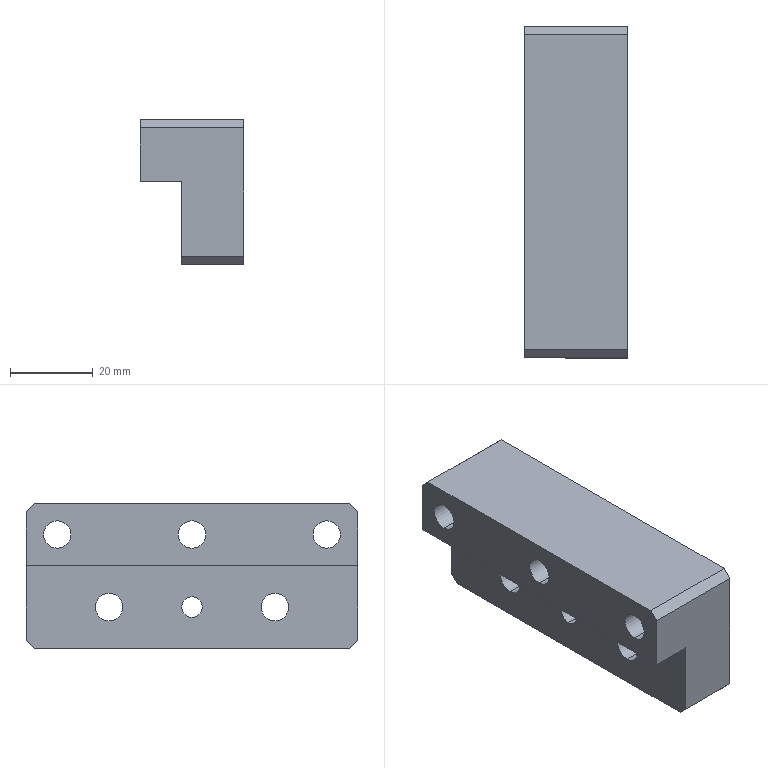Part | SolidWorks | features HoleWzd 3, Chamfer 1, Extrusion 1 | 1 solid | 39 faces | box 25 x 80 x 35 mm | volume 46243 mm3 | cylinder 22 | plane 17 | commonest cylinder face diameters 6.6 x10 11 x10 5 x2
STEP:
#1=CARTESIAN_POINT('',(17.,20.,-19.5));
#2=VERTEX_POINT('',#1);
#3=CARTESIAN_POINT('',(17.,20.,-30.5));
#4=VERTEX_POINT('',#3);
#5=CARTESIAN_POINT('',(17.,20.,-25.));
#6=DIRECTION('',(1.,0.,0.));
#7=DIRECTION('',(0.,0.,-1.));
#8=AXIS2_PLACEMENT_3D('',#5,#6,#7);
#9=CIRCLE('',#8,5.5);
#10=EDGE_CURVE('',#2,#4,#9,.T.);
#11=ORIENTED_EDGE('',*,*,#10,.F.);
#12=CARTESIAN_POINT('',(25.,20.,-19.5));
#13=VERTEX_POINT('',#12);
#14=CARTESIAN_POINT('',(25.,20.,-19.5));
#15=DIRECTION('',(1.,0.,0.));
#16=VECTOR('',#15,1000.);
#17=LINE('',#14,#16);
#18=EDGE_CURVE('',#2,#13,#17,.T.);
#19=ORIENTED_EDGE('',*,*,#18,.T.);
#20=CARTESIAN_POINT('',(25.,20.,-30.5));
#21=VERTEX_POINT('',#20);
#22=CARTESIAN_POINT('',(25.,20.,-25.));
#23=DIRECTION('',(1.,0.,0.));
#24=DIRECTION('',(0.,0.,-1.));
#25=AXIS2_PLACEMENT_3D('',#22,#23,#24);
#26=CIRCLE('',#25,5.5);
#27=EDGE_CURVE('',#13,#21,#26,.T.);
#28=ORIENTED_EDGE('',*,*,#27,.T.);
#29=CARTESIAN_POINT('',(25.,20.,-30.5));
#30=DIRECTION('',(1.,0.,0.));
#31=VECTOR('',#30,1000.);
#32=LINE('',#29,#31);
#33=EDGE_CURVE('',#4,#21,#32,.T.);
#34=ORIENTED_EDGE('',*,*,#33,.F.);
#35=EDGE_LOOP('',(#11,#19,#28,#34));
#36=FACE_OUTER_BOUND('',#35,.T.);
#37=CARTESIAN_POINT('',(25.,20.,-25.));
#38=DIRECTION('',(1.,0.,0.));
#39=DIRECTION('',(0.,0.,-1.));
#40=AXIS2_PLACEMENT_3D('',#37,#38,#39);
#41=CYLINDRICAL_SURFACE('',#40,5.5);
#42=ADVANCED_FACE('',(#36),#41,.F.);
#43=CARTESIAN_POINT('',(10.,20.,-21.7));
#44=VERTEX_POINT('',#43);
#45=CARTESIAN_POINT('',(10.,20.,-28.3));
#46=VERTEX_POINT('',#45);
#47=CARTESIAN_POINT('',(10.,20.,-25.));
#48=DIRECTION('',(1.,0.,0.));
#49=DIRECTION('',(0.,0.,-1.));
#50=AXIS2_PLACEMENT_3D('',#47,#48,#49);
#51=CIRCLE('',#50,3.3);
#52=EDGE_CURVE('',#44,#46,#51,.T.);
#53=ORIENTED_EDGE('',*,*,#52,.F.);
#54=CARTESIAN_POINT('',(17.,20.,-21.7));
#55=VERTEX_POINT('',#54);
#56=CARTESIAN_POINT('',(25.,20.,-21.7));
#57=DIRECTION('',(1.,0.,0.));
#58=VECTOR('',#57,1000.);
#59=LINE('',#56,#58);
#60=EDGE_CURVE('',#44,#55,#59,.T.);
#61=ORIENTED_EDGE('',*,*,#60,.T.);
#62=CARTESIAN_POINT('',(17.,20.,-28.3));
#63=VERTEX_POINT('',#62);
#64=CARTESIAN_POINT('',(17.,20.,-25.));
#65=DIRECTION('',(1.,0.,0.));
#66=DIRECTION('',(0.,0.,-1.));
#67=AXIS2_PLACEMENT_3D('',#64,#65,#66);
#68=CIRCLE('',#67,3.3);
#69=EDGE_CURVE('',#55,#63,#68,.T.);
#70=ORIENTED_EDGE('',*,*,#69,.T.);
#71=CARTESIAN_POINT('',(25.,20.,-28.3));
#72=DIRECTION('',(1.,0.,0.));
#73=VECTOR('',#72,1000.);
#74=LINE('',#71,#73);
#75=EDGE_CURVE('',#46,#63,#74,.T.);
#76=ORIENTED_EDGE('',*,*,#75,.F.);
#77=EDGE_LOOP('',(#53,#61,#70,#76));
#78=FACE_OUTER_BOUND('',#77,.T.);
#79=CARTESIAN_POINT('',(25.,20.,-25.));
#80=DIRECTION('',(1.,0.,0.));
#81=DIRECTION('',(0.,0.,-1.));
#82=AXIS2_PLACEMENT_3D('',#79,#80,#81);
#83=CYLINDRICAL_SURFACE('',#82,3.3);
#84=ADVANCED_FACE('',(#78),#83,.F.);
#85=CARTESIAN_POINT('',(17.,-20.,-19.5));
#86=VERTEX_POINT('',#85);
#87=CARTESIAN_POINT('',(17.,-20.,-30.5));
#88=VERTEX_POINT('',#87);
#89=CARTESIAN_POINT('',(17.,-20.,-25.));
#90=DIRECTION('',(1.,0.,0.));
#91=DIRECTION('',(0.,0.,-1.));
#92=AXIS2_PLACEMENT_3D('',#89,#90,#91);
#93=CIRCLE('',#92,5.5);
#94=EDGE_CURVE('',#86,#88,#93,.T.);
#95=ORIENTED_EDGE('',*,*,#94,.F.);
#96=CARTESIAN_POINT('',(25.,-20.,-19.5));
#97=VERTEX_POINT('',#96);
#98=CARTESIAN_POINT('',(25.,-20.,-19.5));
#99=DIRECTION('',(1.,0.,0.));
#100=VECTOR('',#99,1000.);
#101=LINE('',#98,#100);
#102=EDGE_CURVE('',#86,#97,#101,.T.);
#103=ORIENTED_EDGE('',*,*,#102,.T.);
#104=CARTESIAN_POINT('',(25.,-20.,-30.5));
#105=VERTEX_POINT('',#104);
#106=CARTESIAN_POINT('',(25.,-20.,-25.));
#107=DIRECTION('',(1.,0.,0.));
#108=DIRECTION('',(0.,0.,-1.));
#109=AXIS2_PLACEMENT_3D('',#106,#107,#108);
#110=CIRCLE('',#109,5.5);
#111=EDGE_CURVE('',#97,#105,#110,.T.);
#112=ORIENTED_EDGE('',*,*,#111,.T.);
#113=CARTESIAN_POINT('',(25.,-20.,-30.5));
#114=DIRECTION('',(1.,0.,0.));
#115=VECTOR('',#114,1000.);
#116=LINE('',#113,#115);
#117=EDGE_CURVE('',#88,#105,#116,.T.);
#118=ORIENTED_EDGE('',*,*,#117,.F.);
#119=EDGE_LOOP('',(#95,#103,#112,#118));
#120=FACE_OUTER_BOUND('',#119,.T.);
#121=CARTESIAN_POINT('',(25.,-20.,-25.));
#122=DIRECTION('',(1.,0.,0.));
#123=DIRECTION('',(0.,0.,-1.));
#124=AXIS2_PLACEMENT_3D('',#121,#122,#123);
#125=CYLINDRICAL_SURFACE('',#124,5.5);
#126=ADVANCED_FACE('',(#120),#125,.F.);
#127=CARTESIAN_POINT('',(10.,-20.,-21.7));
#128=VERTEX_POINT('',#127);
#129=CARTESIAN_POINT('',(10.,-20.,-28.3));
#130=VERTEX_POINT('',#129);
#131=CARTESIAN_POINT('',(10.,-20.,-25.));
#132=DIRECTION('',(1.,0.,0.));
#133=DIRECTION('',(0.,0.,-1.));
#134=AXIS2_PLACEMENT_3D('',#131,#132,#133);
#135=CIRCLE('',#134,3.3);
#136=EDGE_CURVE('',#128,#130,#135,.T.);
#137=ORIENTED_EDGE('',*,*,#136,.F.);
#138=CARTESIAN_POINT('',(17.,-20.,-21.7));
#139=VERTEX_POINT('',#138);
#140=CARTESIAN_POINT('',(25.,-20.,-21.7));
#141=DIRECTION('',(1.,0.,0.));
#142=VECTOR('',#141,1000.);
#143=LINE('',#140,#142);
#144=EDGE_CURVE('',#128,#139,#143,.T.);
#145=ORIENTED_EDGE('',*,*,#144,.T.);
#146=CARTESIAN_POINT('',(17.,-20.,-28.3));
#147=VERTEX_POINT('',#146);
#148=CARTESIAN_POINT('',(17.,-20.,-25.));
#149=DIRECTION('',(1.,0.,0.));
#150=DIRECTION('',(0.,0.,-1.));
#151=AXIS2_PLACEMENT_3D('',#148,#149,#150);
#152=CIRCLE('',#151,3.3);
#153=EDGE_CURVE('',#139,#147,#152,.T.);
#154=ORIENTED_EDGE('',*,*,#153,.T.);
#155=CARTESIAN_POINT('',(25.,-20.,-28.3));
#156=DIRECTION('',(1.,0.,0.));
#157=VECTOR('',#156,1000.);
#158=LINE('',#155,#157);
#159=EDGE_CURVE('',#130,#147,#158,.T.);
#160=ORIENTED_EDGE('',*,*,#159,.F.);
#161=EDGE_LOOP('',(#137,#145,#154,#160));
#162=FACE_OUTER_BOUND('',#161,.T.);
#163=CARTESIAN_POINT('',(25.,-20.,-25.));
#164=DIRECTION('',(1.,0.,0.));
#165=DIRECTION('',(0.,0.,-1.));
#166=AXIS2_PLACEMENT_3D('',#163,#164,#165);
#167=CYLINDRICAL_SURFACE('',#166,3.3);
#168=ADVANCED_FACE('',(#162),#167,.F.);
#169=CARTESIAN_POINT('',(10.,0.,-22.5));
#170=VERTEX_POINT('',#169);
#171=CARTESIAN_POINT('',(10.,0.,-27.5));
#172=VERTEX_POINT('',#171);
#173=CARTESIAN_POINT('',(10.,0.,-25.));
#174=DIRECTION('',(1.,0.,0.));
#175=DIRECTION('',(0.,0.,-1.));
#176=AXIS2_PLACEMENT_3D('',#173,#174,#175);
#177=CIRCLE('',#176,2.5);
#178=EDGE_CURVE('',#170,#172,#177,.T.);
#179=ORIENTED_EDGE('',*,*,#178,.F.);
#180=CARTESIAN_POINT('',(25.,0.,-22.5));
#181=VERTEX_POINT('',#180);
#182=CARTESIAN_POINT('',(25.,0.,-22.5));
#183=DIRECTION('',(1.,0.,0.));
#184=VECTOR('',#183,1000.);
#185=LINE('',#182,#184);
#186=EDGE_CURVE('',#170,#181,#185,.T.);
#187=ORIENTED_EDGE('',*,*,#186,.T.);
#188=CARTESIAN_POINT('',(25.,0.,-27.5));
#189=VERTEX_POINT('',#188);
#190=CARTESIAN_POINT('',(25.,0.,-25.));
#191=DIRECTION('',(1.,0.,0.));
#192=DIRECTION('',(0.,0.,-1.));
#193=AXIS2_PLACEMENT_3D('',#190,#191,#192);
#194=CIRCLE('',#193,2.5);
#195=EDGE_CURVE('',#181,#189,#194,.T.);
#196=ORIENTED_EDGE('',*,*,#195,.T.);
#197=CARTESIAN_POINT('',(25.,0.,-27.5));
#198=DIRECTION('',(1.,0.,0.));
#199=VECTOR('',#198,1000.);
#200=LINE('',#197,#199);
#201=EDGE_CURVE('',#172,#189,#200,.T.);
#202=ORIENTED_EDGE('',*,*,#201,.F.);
#203=EDGE_LOOP('',(#179,#187,#196,#202));
#204=FACE_OUTER_BOUND('',#203,.T.);
#205=CARTESIAN_POINT('',(25.,0.,-25.));
#206=DIRECTION('',(1.,0.,0.));
#207=DIRECTION('',(0.,0.,-1.));
#208=AXIS2_PLACEMENT_3D('',#205,#206,#207);
#209=CYLINDRICAL_SURFACE('',#208,2.5);
#210=ADVANCED_FACE('',(#204),#209,.F.);
#211=CARTESIAN_POINT('',(10.,32.5,-2.));
#212=VERTEX_POINT('',#211);
#213=CARTESIAN_POINT('',(10.,32.5,-13.));
#214=VERTEX_POINT('',#213);
#215=CARTESIAN_POINT('',(10.,32.5,-7.5));
#216=DIRECTION('',(1.,0.,0.));
#217=DIRECTION('',(0.,0.,-1.));
#218=AXIS2_PLACEMENT_3D('',#215,#216,#217);
#219=CIRCLE('',#218,5.5);
#220=EDGE_CURVE('',#212,#214,#219,.T.);
#221=ORIENTED_EDGE('',*,*,#220,.F.);
#222=CARTESIAN_POINT('',(25.,32.5,-2.));
#223=VERTEX_POINT('',#222);
#224=CARTESIAN_POINT('',(25.,32.5,-2.));
#225=DIRECTION('',(1.,0.,0.));
#226=VECTOR('',#225,1000.);
#227=LINE('',#224,#226);
#228=EDGE_CURVE('',#212,#223,#227,.T.);
#229=ORIENTED_EDGE('',*,*,#228,.T.);
#230=CARTESIAN_POINT('',(25.,32.5,-13.));
#231=VERTEX_POINT('',#230);
#232=CARTESIAN_POINT('',(25.,32.5,-7.5));
#233=DIRECTION('',(1.,0.,0.));
#234=DIRECTION('',(0.,0.,-1.));
#235=AXIS2_PLACEMENT_3D('',#232,#233,#234);
#236=CIRCLE('',#235,5.5);
#237=EDGE_CURVE('',#223,#231,#236,.T.);
#238=ORIENTED_EDGE('',*,*,#237,.T.);
#239=CARTESIAN_POINT('',(25.,32.5,-13.));
#240=DIRECTION('',(1.,0.,0.));
#241=VECTOR('',#240,1000.);
#242=LINE('',#239,#241);
#243=EDGE_CURVE('',#214,#231,#242,.T.);
#244=ORIENTED_EDGE('',*,*,#243,.F.);
#245=EDGE_LOOP('',(#221,#229,#238,#244));
#246=FACE_OUTER_BOUND('',#245,.T.);
#247=CARTESIAN_POINT('',(25.,32.5,-7.5));
#248=DIRECTION('',(1.,0.,0.));
#249=DIRECTION('',(0.,0.,-1.));
#250=AXIS2_PLACEMENT_3D('',#247,#248,#249);
#251=CYLINDRICAL_SURFACE('',#250,5.5);
#252=ADVANCED_FACE('',(#246),#251,.F.);
#253=CARTESIAN_POINT('',(0.,32.5,-4.2));
#254=VERTEX_POINT('',#253);
#255=CARTESIAN_POINT('',(0.,32.5,-10.8));
#256=VERTEX_POINT('',#255);
#257=CARTESIAN_POINT('',(0.,32.5,-7.5));
#258=DIRECTION('',(1.,0.,0.));
#259=DIRECTION('',(0.,0.,-1.));
#260=AXIS2_PLACEMENT_3D('',#257,#258,#259);
#261=CIRCLE('',#260,3.3);
#262=EDGE_CURVE('',#254,#256,#261,.T.);
#263=ORIENTED_EDGE('',*,*,#262,.F.);
#264=CARTESIAN_POINT('',(10.,32.5,-4.2));
#265=VERTEX_POINT('',#264);
#266=CARTESIAN_POINT('',(25.,32.5,-4.2));
#267=DIRECTION('',(1.,0.,0.));
#268=VECTOR('',#267,1000.);
#269=LINE('',#266,#268);
#270=EDGE_CURVE('',#254,#265,#269,.T.);
#271=ORIENTED_EDGE('',*,*,#270,.T.);
#272=CARTESIAN_POINT('',(10.,32.5,-10.8));
#273=VERTEX_POINT('',#272);
#274=CARTESIAN_POINT('',(10.,32.5,-7.5));
#275=DIRECTION('',(1.,0.,0.));
#276=DIRECTION('',(0.,0.,-1.));
#277=AXIS2_PLACEMENT_3D('',#274,#275,#276);
#278=CIRCLE('',#277,3.3);
#279=EDGE_CURVE('',#265,#273,#278,.T.);
#280=ORIENTED_EDGE('',*,*,#279,.T.);
#281=CARTESIAN_POINT('',(25.,32.5,-10.8));
#282=DIRECTION('',(1.,0.,0.));
#283=VECTOR('',#282,1000.);
#284=LINE('',#281,#283);
#285=EDGE_CURVE('',#256,#273,#284,.T.);
#286=ORIENTED_EDGE('',*,*,#285,.F.);
#287=EDGE_LOOP('',(#263,#271,#280,#286));
#288=FACE_OUTER_BOUND('',#287,.T.);
#289=CARTESIAN_POINT('',(25.,32.5,-7.5));
#290=DIRECTION('',(1.,0.,0.));
#291=DIRECTION('',(0.,0.,-1.));
#292=AXIS2_PLACEMENT_3D('',#289,#290,#291);
#293=CYLINDRICAL_SURFACE('',#292,3.3);
#294=ADVANCED_FACE('',(#288),#293,.F.);
#295=CARTESIAN_POINT('',(10.,0.,-2.));
#296=VERTEX_POINT('',#295);
#297=CARTESIAN_POINT('',(10.,0.,-13.));
#298=VERTEX_POINT('',#297);
#299=CARTESIAN_POINT('',(10.,0.,-7.5));
#300=DIRECTION('',(1.,0.,0.));
#301=DIRECTION('',(0.,0.,-1.));
#302=AXIS2_PLACEMENT_3D('',#299,#300,#301);
#303=CIRCLE('',#302,5.5);
#304=EDGE_CURVE('',#296,#298,#303,.T.);
#305=ORIENTED_EDGE('',*,*,#304,.F.);
#306=CARTESIAN_POINT('',(25.,0.,-2.));
#307=VERTEX_POINT('',#306);
#308=CARTESIAN_POINT('',(25.,0.,-2.));
#309=DIRECTION('',(1.,0.,0.));
#310=VECTOR('',#309,1000.);
#311=LINE('',#308,#310);
#312=EDGE_CURVE('',#296,#307,#311,.T.);
#313=ORIENTED_EDGE('',*,*,#312,.T.);
#314=CARTESIAN_POINT('',(25.,0.,-13.));
#315=VERTEX_POINT('',#314);
#316=CARTESIAN_POINT('',(25.,0.,-7.5));
#317=DIRECTION('',(1.,0.,0.));
#318=DIRECTION('',(0.,0.,-1.));
#319=AXIS2_PLACEMENT_3D('',#316,#317,#318);
#320=CIRCLE('',#319,5.5);
#321=EDGE_CURVE('',#307,#315,#320,.T.);
#322=ORIENTED_EDGE('',*,*,#321,.T.);
#323=CARTESIAN_POINT('',(25.,0.,-13.));
#324=DIRECTION('',(1.,0.,0.));
#325=VECTOR('',#324,1000.);
#326=LINE('',#323,#325);
#327=EDGE_CURVE('',#298,#315,#326,.T.);
#328=ORIENTED_EDGE('',*,*,#327,.F.);
#329=EDGE_LOOP('',(#305,#313,#322,#328));
#330=FACE_OUTER_BOUND('',#329,.T.);
#331=CARTESIAN_POINT('',(25.,0.,-7.5));
#332=DIRECTION('',(1.,0.,0.));
#333=DIRECTION('',(0.,0.,-1.));
#334=AXIS2_PLACEMENT_3D('',#331,#332,#333);
#335=CYLINDRICAL_SURFACE('',#334,5.5);
#336=ADVANCED_FACE('',(#330),#335,.F.);
#337=CARTESIAN_POINT('',(0.,0.,-4.2));
#338=VERTEX_POINT('',#337);
#339=CARTESIAN_POINT('',(0.,0.,-10.8));
#340=VERTEX_POINT('',#339);
#341=CARTESIAN_POINT('',(0.,0.,-7.5));
#342=DIRECTION('',(1.,0.,0.));
#343=DIRECTION('',(0.,0.,-1.));
#344=AXIS2_PLACEMENT_3D('',#341,#342,#343);
#345=CIRCLE('',#344,3.3);
#346=EDGE_CURVE('',#338,#340,#345,.T.);
#347=ORIENTED_EDGE('',*,*,#346,.F.);
#348=CARTESIAN_POINT('',(10.,0.,-4.2));
#349=VERTEX_POINT('',#348);
#350=CARTESIAN_POINT('',(25.,0.,-4.2));
#351=DIRECTION('',(1.,0.,0.));
#352=VECTOR('',#351,1000.);
#353=LINE('',#350,#352);
#354=EDGE_CURVE('',#338,#349,#353,.T.);
#355=ORIENTED_EDGE('',*,*,#354,.T.);
#356=CARTESIAN_POINT('',(10.,0.,-10.8));
#357=VERTEX_POINT('',#356);
#358=CARTESIAN_POINT('',(10.,0.,-7.5));
#359=DIRECTION('',(1.,0.,0.));
#360=DIRECTION('',(0.,0.,-1.));
#361=AXIS2_PLACEMENT_3D('',#358,#359,#360);
#362=CIRCLE('',#361,3.3);
#363=EDGE_CURVE('',#349,#357,#362,.T.);
#364=ORIENTED_EDGE('',*,*,#363,.T.);
#365=CARTESIAN_POINT('',(25.,0.,-10.8));
#366=DIRECTION('',(1.,0.,0.));
#367=VECTOR('',#366,1000.);
#368=LINE('',#365,#367);
#369=EDGE_CURVE('',#340,#357,#368,.T.);
#370=ORIENTED_EDGE('',*,*,#369,.F.);
#371=EDGE_LOOP('',(#347,#355,#364,#370));
#372=FACE_OUTER_BOUND('',#371,.T.);
#373=CARTESIAN_POINT('',(25.,0.,-7.5));
#374=DIRECTION('',(1.,0.,0.));
#375=DIRECTION('',(0.,0.,-1.));
#376=AXIS2_PLACEMENT_3D('',#373,#374,#375);
#377=CYLINDRICAL_SURFACE('',#376,3.3);
#378=ADVANCED_FACE('',(#372),#377,.F.);
#379=CARTESIAN_POINT('',(10.,-32.5,-2.));
#380=VERTEX_POINT('',#379);
#381=CARTESIAN_POINT('',(10.,-32.5,-13.));
#382=VERTEX_POINT('',#381);
#383=CARTESIAN_POINT('',(10.,-32.5,-7.5));
#384=DIRECTION('',(1.,0.,0.));
#385=DIRECTION('',(0.,0.,-1.));
#386=AXIS2_PLACEMENT_3D('',#383,#384,#385);
#387=CIRCLE('',#386,5.5);
#388=EDGE_CURVE('',#380,#382,#387,.T.);
#389=ORIENTED_EDGE('',*,*,#388,.F.);
#390=CARTESIAN_POINT('',(25.,-32.5,-2.));
#391=VERTEX_POINT('',#390);
#392=CARTESIAN_POINT('',(25.,-32.5,-2.));
#393=DIRECTION('',(1.,0.,0.));
#394=VECTOR('',#393,1000.);
#395=LINE('',#392,#394);
#396=EDGE_CURVE('',#380,#391,#395,.T.);
#397=ORIENTED_EDGE('',*,*,#396,.T.);
#398=CARTESIAN_POINT('',(25.,-32.5,-13.));
#399=VERTEX_POINT('',#398);
#400=CARTESIAN_POINT('',(25.,-32.5,-7.5));
#401=DIRECTION('',(1.,0.,0.));
#402=DIRECTION('',(0.,0.,-1.));
#403=AXIS2_PLACEMENT_3D('',#400,#401,#402);
#404=CIRCLE('',#403,5.5);
#405=EDGE_CURVE('',#391,#399,#404,.T.);
#406=ORIENTED_EDGE('',*,*,#405,.T.);
#407=CARTESIAN_POINT('',(25.,-32.5,-13.));
#408=DIRECTION('',(1.,0.,0.));
#409=VECTOR('',#408,1000.);
#410=LINE('',#407,#409);
#411=EDGE_CURVE('',#382,#399,#410,.T.);
#412=ORIENTED_EDGE('',*,*,#411,.F.);
#413=EDGE_LOOP('',(#389,#397,#406,#412));
#414=FACE_OUTER_BOUND('',#413,.T.);
#415=CARTESIAN_POINT('',(25.,-32.5,-7.5));
#416=DIRECTION('',(1.,0.,0.));
#417=DIRECTION('',(0.,0.,-1.));
#418=AXIS2_PLACEMENT_3D('',#415,#416,#417);
#419=CYLINDRICAL_SURFACE('',#418,5.5);
#420=ADVANCED_FACE('',(#414),#419,.F.);
#421=CARTESIAN_POINT('',(0.,-32.5,-4.2));
#422=VERTEX_POINT('',#421);
#423=CARTESIAN_POINT('',(0.,-32.5,-10.8));
#424=VERTEX_POINT('',#423);
#425=CARTESIAN_POINT('',(0.,-32.5,-7.5));
#426=DIRECTION('',(1.,0.,0.));
#427=DIRECTION('',(0.,0.,-1.));
#428=AXIS2_PLACEMENT_3D('',#425,#426,#427);
#429=CIRCLE('',#428,3.3);
#430=EDGE_CURVE('',#422,#424,#429,.T.);
#431=ORIENTED_EDGE('',*,*,#430,.F.);
#432=CARTESIAN_POINT('',(10.,-32.5,-4.2));
#433=VERTEX_POINT('',#432);
#434=CARTESIAN_POINT('',(25.,-32.5,-4.2));
#435=DIRECTION('',(1.,0.,0.));
#436=VECTOR('',#435,1000.);
#437=LINE('',#434,#436);
#438=EDGE_CURVE('',#422,#433,#437,.T.);
#439=ORIENTED_EDGE('',*,*,#438,.T.);
#440=CARTESIAN_POINT('',(10.,-32.5,-10.8));
#441=VERTEX_POINT('',#440);
#442=CARTESIAN_POINT('',(10.,-32.5,-7.5));
#443=DIRECTION('',(1.,0.,0.));
#444=DIRECTION('',(0.,0.,-1.));
#445=AXIS2_PLACEMENT_3D('',#442,#443,#444);
#446=CIRCLE('',#445,3.3);
#447=EDGE_CURVE('',#433,#441,#446,.T.);
#448=ORIENTED_EDGE('',*,*,#447,.T.);
#449=CARTESIAN_POINT('',(25.,-32.5,-10.8));
#450=DIRECTION('',(1.,0.,0.));
#451=VECTOR('',#450,1000.);
#452=LINE('',#449,#451);
#453=EDGE_CURVE('',#424,#441,#452,.T.);
#454=ORIENTED_EDGE('',*,*,#453,.F.);
#455=EDGE_LOOP('',(#431,#439,#448,#454));
#456=FACE_OUTER_BOUND('',#455,.T.);
#457=CARTESIAN_POINT('',(25.,-32.5,-7.5));
#458=DIRECTION('',(1.,0.,0.));
#459=DIRECTION('',(0.,0.,-1.));
#460=AXIS2_PLACEMENT_3D('',#457,#458,#459);
#461=CYLINDRICAL_SURFACE('',#460,3.3);
#462=ADVANCED_FACE('',(#456),#461,.F.);
#463=CARTESIAN_POINT('',(25.,20.,-25.));
#464=DIRECTION('',(1.,0.,0.));
#465=DIRECTION('',(0.,0.,-1.));
#466=AXIS2_PLACEMENT_3D('',#463,#464,#465);
#467=CIRCLE('',#466,5.5);
#468=EDGE_CURVE('',#21,#13,#467,.T.);
#469=ORIENTED_EDGE('',*,*,#468,.F.);
#470=ORIENTED_EDGE('',*,*,#27,.F.);
#471=EDGE_LOOP('',(#469,#470));
#472=FACE_BOUND('',#471,.T.);
#473=CARTESIAN_POINT('',(25.,0.,-25.));
#474=DIRECTION('',(1.,0.,0.));
#475=DIRECTION('',(0.,0.,-1.));
#476=AXIS2_PLACEMENT_3D('',#473,#474,#475);
#477=CIRCLE('',#476,2.5);
#478=EDGE_CURVE('',#189,#181,#477,.T.);
#479=ORIENTED_EDGE('',*,*,#478,.F.);
#480=ORIENTED_EDGE('',*,*,#195,.F.);
#481=EDGE_LOOP('',(#479,#480));
#482=FACE_BOUND('',#481,.T.);
#483=CARTESIAN_POINT('',(25.,-32.5,-7.5));
#484=DIRECTION('',(1.,0.,0.));
#485=DIRECTION('',(0.,0.,-1.));
#486=AXIS2_PLACEMENT_3D('',#483,#484,#485);
#487=CIRCLE('',#486,5.5);
#488=EDGE_CURVE('',#399,#391,#487,.T.);
#489=ORIENTED_EDGE('',*,*,#488,.F.);
#490=ORIENTED_EDGE('',*,*,#405,.F.);
#491=EDGE_LOOP('',(#489,#490));
#492=FACE_BOUND('',#491,.T.);
#493=CARTESIAN_POINT('',(25.,38.,0.));
#494=VERTEX_POINT('',#493);
#495=CARTESIAN_POINT('',(25.,-38.,0.));
#496=VERTEX_POINT('',#495);
#497=CARTESIAN_POINT('',(25.,40.,0.));
#498=DIRECTION('',(0.,-1.,0.));
#499=VECTOR('',#498,1000.);
#500=LINE('',#497,#499);
#501=EDGE_CURVE('',#494,#496,#500,.T.);
#502=ORIENTED_EDGE('',*,*,#501,.T.);
#503=CARTESIAN_POINT('',(25.,-40.,-2.));
#504=VERTEX_POINT('',#503);
#505=CARTESIAN_POINT('',(25.,-38.,0.));
#506=DIRECTION('',(0.,-0.7071,-0.7071));
#507=VECTOR('',#506,1000.);
#508=LINE('',#505,#507);
#509=EDGE_CURVE('',#496,#504,#508,.T.);
#510=ORIENTED_EDGE('',*,*,#509,.T.);
#511=CARTESIAN_POINT('',(25.,-40.,-33.));
#512=VERTEX_POINT('',#511);
#513=CARTESIAN_POINT('',(25.,-40.,0.));
#514=DIRECTION('',(0.,0.,-1.));
#515=VECTOR('',#514,1000.);
#516=LINE('',#513,#515);
#517=EDGE_CURVE('',#504,#512,#516,.T.);
#518=ORIENTED_EDGE('',*,*,#517,.T.);
#519=CARTESIAN_POINT('',(25.,-38.,-35.));
#520=VERTEX_POINT('',#519);
#521=CARTESIAN_POINT('',(25.,-38.,-35.));
#522=DIRECTION('',(0.,0.7071,-0.7071));
#523=VECTOR('',#522,1000.);
#524=LINE('',#521,#523);
#525=EDGE_CURVE('',#512,#520,#524,.T.);
#526=ORIENTED_EDGE('',*,*,#525,.T.);
#527=CARTESIAN_POINT('',(25.,38.,-35.));
#528=VERTEX_POINT('',#527);
#529=CARTESIAN_POINT('',(25.,40.,-35.));
#530=DIRECTION('',(0.,-1.,0.));
#531=VECTOR('',#530,1000.);
#532=LINE('',#529,#531);
#533=EDGE_CURVE('',#528,#520,#532,.T.);
#534=ORIENTED_EDGE('',*,*,#533,.F.);
#535=CARTESIAN_POINT('',(25.,40.,-33.));
#536=VERTEX_POINT('',#535);
#537=CARTESIAN_POINT('',(25.,40.,-33.));
#538=DIRECTION('',(0.,0.7071,0.7071));
#539=VECTOR('',#538,1000.);
#540=LINE('',#537,#539);
#541=EDGE_CURVE('',#528,#536,#540,.T.);
#542=ORIENTED_EDGE('',*,*,#541,.T.);
#543=CARTESIAN_POINT('',(25.,40.,-2.));
#544=VERTEX_POINT('',#543);
#545=CARTESIAN_POINT('',(25.,40.,0.));
#546=DIRECTION('',(0.,0.,-1.));
#547=VECTOR('',#546,1000.);
#548=LINE('',#545,#547);
#549=EDGE_CURVE('',#544,#536,#548,.T.);
#550=ORIENTED_EDGE('',*,*,#549,.F.);
#551=CARTESIAN_POINT('',(25.,40.,-2.));
#552=DIRECTION('',(0.,-0.7071,0.7071));
#553=VECTOR('',#552,1000.);
#554=LINE('',#551,#553);
#555=EDGE_CURVE('',#544,#494,#554,.T.);
#556=ORIENTED_EDGE('',*,*,#555,.T.);
#557=EDGE_LOOP('',(#502,#510,#518,#526,#534,#542,#550,#556));
#558=FACE_OUTER_BOUND('',#557,.T.);
#559=CARTESIAN_POINT('',(25.,0.,-7.5));
#560=DIRECTION('',(1.,0.,0.));
#561=DIRECTION('',(0.,0.,-1.));
#562=AXIS2_PLACEMENT_3D('',#559,#560,#561);
#563=CIRCLE('',#562,5.5);
#564=EDGE_CURVE('',#315,#307,#563,.T.);
#565=ORIENTED_EDGE('',*,*,#564,.F.);
#566=ORIENTED_EDGE('',*,*,#321,.F.);
#567=EDGE_LOOP('',(#565,#566));
#568=FACE_BOUND('',#567,.T.);
#569=CARTESIAN_POINT('',(25.,32.5,-7.5));
#570=DIRECTION('',(1.,0.,0.));
#571=DIRECTION('',(0.,0.,-1.));
#572=AXIS2_PLACEMENT_3D('',#569,#570,#571);
#573=CIRCLE('',#572,5.5);
#574=EDGE_CURVE('',#231,#223,#573,.T.);
#575=ORIENTED_EDGE('',*,*,#574,.F.);
#576=ORIENTED_EDGE('',*,*,#237,.F.);
#577=EDGE_LOOP('',(#575,#576));
#578=FACE_BOUND('',#577,.T.);
#579=CARTESIAN_POINT('',(25.,-20.,-25.));
#580=DIRECTION('',(1.,0.,0.));
#581=DIRECTION('',(0.,0.,-1.));
#582=AXIS2_PLACEMENT_3D('',#579,#580,#581);
#583=CIRCLE('',#582,5.5);
#584=EDGE_CURVE('',#105,#97,#583,.T.);
#585=ORIENTED_EDGE('',*,*,#584,.F.);
#586=ORIENTED_EDGE('',*,*,#111,.F.);
#587=EDGE_LOOP('',(#585,#586));
#588=FACE_BOUND('',#587,.T.);
#589=CARTESIAN_POINT('',(25.,40.,0.));
#590=DIRECTION('',(-1.,0.,0.));
#591=DIRECTION('',(0.,0.,1.));
#592=AXIS2_PLACEMENT_3D('',#589,#590,#591);
#593=PLANE('',#592);
#594=ADVANCED_FACE('',(#472,#482,#492,#558,#568,#578,#588),#593,.F.);
#595=CARTESIAN_POINT('',(0.,32.5,-7.5));
#596=DIRECTION('',(1.,0.,0.));
#597=DIRECTION('',(0.,0.,-1.));
#598=AXIS2_PLACEMENT_3D('',#595,#596,#597);
#599=CIRCLE('',#598,3.3);
#600=EDGE_CURVE('',#256,#254,#599,.T.);
#601=ORIENTED_EDGE('',*,*,#600,.T.);
#602=ORIENTED_EDGE('',*,*,#262,.T.);
#603=EDGE_LOOP('',(#601,#602));
#604=FACE_BOUND('',#603,.T.);
#605=CARTESIAN_POINT('',(0.,0.,-7.5));
#606=DIRECTION('',(1.,0.,0.));
#607=DIRECTION('',(0.,0.,-1.));
#608=AXIS2_PLACEMENT_3D('',#605,#606,#607);
#609=CIRCLE('',#608,3.3);
#610=EDGE_CURVE('',#340,#338,#609,.T.);
#611=ORIENTED_EDGE('',*,*,#610,.T.);
#612=ORIENTED_EDGE('',*,*,#346,.T.);
#613=EDGE_LOOP('',(#611,#612));
#614=FACE_BOUND('',#613,.T.);
#615=CARTESIAN_POINT('',(0.,-32.5,-7.5));
#616=DIRECTION('',(1.,0.,0.));
#617=DIRECTION('',(0.,0.,-1.));
#618=AXIS2_PLACEMENT_3D('',#615,#616,#617);
#619=CIRCLE('',#618,3.3);
#620=EDGE_CURVE('',#424,#422,#619,.T.);
#621=ORIENTED_EDGE('',*,*,#620,.T.);
#622=ORIENTED_EDGE('',*,*,#430,.T.);
#623=EDGE_LOOP('',(#621,#622));
#624=FACE_BOUND('',#623,.T.);
#625=CARTESIAN_POINT('',(0.,-40.,-15.));
#626=VERTEX_POINT('',#625);
#627=CARTESIAN_POINT('',(0.,-40.,-2.));
#628=VERTEX_POINT('',#627);
#629=CARTESIAN_POINT('',(0.,-40.,-15.));
#630=DIRECTION('',(0.,0.,1.));
#631=VECTOR('',#630,1000.);
#632=LINE('',#629,#631);
#633=EDGE_CURVE('',#626,#628,#632,.T.);
#634=ORIENTED_EDGE('',*,*,#633,.T.);
#635=CARTESIAN_POINT('',(0.,-38.,0.));
#636=VERTEX_POINT('',#635);
#637=CARTESIAN_POINT('',(0.,-38.,0.));
#638=DIRECTION('',(0.,0.7071,0.7071));
#639=VECTOR('',#638,1000.);
#640=LINE('',#637,#639);
#641=EDGE_CURVE('',#628,#636,#640,.T.);
#642=ORIENTED_EDGE('',*,*,#641,.T.);
#643=CARTESIAN_POINT('',(0.,38.,0.));
#644=VERTEX_POINT('',#643);
#645=CARTESIAN_POINT('',(0.,40.,0.));
#646=DIRECTION('',(0.,-1.,0.));
#647=VECTOR('',#646,1000.);
#648=LINE('',#645,#647);
#649=EDGE_CURVE('',#644,#636,#648,.T.);
#650=ORIENTED_EDGE('',*,*,#649,.F.);
#651=CARTESIAN_POINT('',(0.,40.,-2.));
#652=VERTEX_POINT('',#651);
#653=CARTESIAN_POINT('',(0.,40.,-2.));
#654=DIRECTION('',(0.,0.7071,-0.7071));
#655=VECTOR('',#654,1000.);
#656=LINE('',#653,#655);
#657=EDGE_CURVE('',#644,#652,#656,.T.);
#658=ORIENTED_EDGE('',*,*,#657,.T.);
#659=CARTESIAN_POINT('',(0.,40.,-15.));
#660=VERTEX_POINT('',#659);
#661=CARTESIAN_POINT('',(0.,40.,-15.));
#662=DIRECTION('',(0.,0.,1.));
#663=VECTOR('',#662,1000.);
#664=LINE('',#661,#663);
#665=EDGE_CURVE('',#660,#652,#664,.T.);
#666=ORIENTED_EDGE('',*,*,#665,.F.);
#667=CARTESIAN_POINT('',(0.,40.,-15.));
#668=DIRECTION('',(0.,-1.,0.));
#669=VECTOR('',#668,1000.);
#670=LINE('',#667,#669);
#671=EDGE_CURVE('',#660,#626,#670,.T.);
#672=ORIENTED_EDGE('',*,*,#671,.T.);
#673=EDGE_LOOP('',(#634,#642,#650,#658,#666,#672));
#674=FACE_OUTER_BOUND('',#673,.T.);
#675=CARTESIAN_POINT('',(0.,40.,-15.));
#676=DIRECTION('',(1.,0.,0.));
#677=DIRECTION('',(0.,0.,-1.));
#678=AXIS2_PLACEMENT_3D('',#675,#676,#677);
#679=PLANE('',#678);
#680=ADVANCED_FACE('',(#604,#614,#624,#674),#679,.F.);
#681=ORIENTED_EDGE('',*,*,#649,.T.);
#682=CARTESIAN_POINT('',(0.,-38.,0.));
#683=DIRECTION('',(1.,0.,0.));
#684=VECTOR('',#683,1000.);
#685=LINE('',#682,#684);
#686=EDGE_CURVE('',#636,#496,#685,.T.);
#687=ORIENTED_EDGE('',*,*,#686,.T.);
#688=ORIENTED_EDGE('',*,*,#501,.F.);
#689=CARTESIAN_POINT('',(0.,38.,0.));
#690=DIRECTION('',(-1.,0.,0.));
#691=VECTOR('',#690,1000.);
#692=LINE('',#689,#691);
#693=EDGE_CURVE('',#494,#644,#692,.T.);
#694=ORIENTED_EDGE('',*,*,#693,.T.);
#695=EDGE_LOOP('',(#681,#687,#688,#694));
#696=FACE_OUTER_BOUND('',#695,.T.);
#697=CARTESIAN_POINT('',(0.,40.,0.));
#698=DIRECTION('',(0.,0.,-1.));
#699=DIRECTION('',(-1.,0.,0.));
#700=AXIS2_PLACEMENT_3D('',#697,#698,#699);
#701=PLANE('',#700);
#702=ADVANCED_FACE('',(#696),#701,.F.);
#703=ORIENTED_EDGE('',*,*,#533,.T.);
#704=CARTESIAN_POINT('',(10.,-38.,-35.));
#705=VERTEX_POINT('',#704);
#706=CARTESIAN_POINT('',(25.,-38.,-35.));
#707=DIRECTION('',(-1.,0.,0.));
#708=VECTOR('',#707,1000.);
#709=LINE('',#706,#708);
#710=EDGE_CURVE('',#520,#705,#709,.T.);
#711=ORIENTED_EDGE('',*,*,#710,.T.);
#712=CARTESIAN_POINT('',(10.,38.,-35.));
#713=VERTEX_POINT('',#712);
#714=CARTESIAN_POINT('',(10.,40.,-35.));
#715=DIRECTION('',(0.,-1.,0.));
#716=VECTOR('',#715,1000.);
#717=LINE('',#714,#716);
#718=EDGE_CURVE('',#713,#705,#717,.T.);
#719=ORIENTED_EDGE('',*,*,#718,.F.);
#720=CARTESIAN_POINT('',(25.,38.,-35.));
#721=DIRECTION('',(1.,0.,0.));
#722=VECTOR('',#721,1000.);
#723=LINE('',#720,#722);
#724=EDGE_CURVE('',#713,#528,#723,.T.);
#725=ORIENTED_EDGE('',*,*,#724,.T.);
#726=EDGE_LOOP('',(#703,#711,#719,#725));
#727=FACE_OUTER_BOUND('',#726,.T.);
#728=CARTESIAN_POINT('',(25.,40.,-35.));
#729=DIRECTION('',(0.,0.,1.));
#730=DIRECTION('',(1.,0.,0.));
#731=AXIS2_PLACEMENT_3D('',#728,#729,#730);
#732=PLANE('',#731);
#733=ADVANCED_FACE('',(#727),#732,.F.);
#734=CARTESIAN_POINT('',(10.,20.,-25.));
#735=DIRECTION('',(1.,0.,0.));
#736=DIRECTION('',(0.,0.,-1.));
#737=AXIS2_PLACEMENT_3D('',#734,#735,#736);
#738=CIRCLE('',#737,3.3);
#739=EDGE_CURVE('',#46,#44,#738,.T.);
#740=ORIENTED_EDGE('',*,*,#739,.T.);
#741=ORIENTED_EDGE('',*,*,#52,.T.);
#742=EDGE_LOOP('',(#740,#741));
#743=FACE_BOUND('',#742,.T.);
#744=CARTESIAN_POINT('',(10.,-20.,-25.));
#745=DIRECTION('',(1.,0.,0.));
#746=DIRECTION('',(0.,0.,-1.));
#747=AXIS2_PLACEMENT_3D('',#744,#745,#746);
#748=CIRCLE('',#747,3.3);
#749=EDGE_CURVE('',#130,#128,#748,.T.);
#750=ORIENTED_EDGE('',*,*,#749,.T.);
#751=ORIENTED_EDGE('',*,*,#136,.T.);
#752=EDGE_LOOP('',(#750,#751));
#753=FACE_BOUND('',#752,.T.);
#754=CARTESIAN_POINT('',(10.,0.,-25.));
#755=DIRECTION('',(1.,0.,0.));
#756=DIRECTION('',(0.,0.,-1.));
#757=AXIS2_PLACEMENT_3D('',#754,#755,#756);
#758=CIRCLE('',#757,2.5);
#759=EDGE_CURVE('',#172,#170,#758,.T.);
#760=ORIENTED_EDGE('',*,*,#759,.T.);
#761=ORIENTED_EDGE('',*,*,#178,.T.);
#762=EDGE_LOOP('',(#760,#761));
#763=FACE_BOUND('',#762,.T.);
#764=ORIENTED_EDGE('',*,*,#718,.T.);
#765=CARTESIAN_POINT('',(10.,-40.,-33.));
#766=VERTEX_POINT('',#765);
#767=CARTESIAN_POINT('',(10.,-38.,-35.));
#768=DIRECTION('',(0.,-0.7071,0.7071));
#769=VECTOR('',#768,1000.);
#770=LINE('',#767,#769);
#771=EDGE_CURVE('',#705,#766,#770,.T.);
#772=ORIENTED_EDGE('',*,*,#771,.T.);
#773=CARTESIAN_POINT('',(10.,-40.,-15.));
#774=VERTEX_POINT('',#773);
#775=CARTESIAN_POINT('',(10.,-40.,-35.));
#776=DIRECTION('',(0.,0.,1.));
#777=VECTOR('',#776,1000.);
#778=LINE('',#775,#777);
#779=EDGE_CURVE('',#766,#774,#778,.T.);
#780=ORIENTED_EDGE('',*,*,#779,.T.);
#781=CARTESIAN_POINT('',(10.,40.,-15.));
#782=VERTEX_POINT('',#781);
#783=CARTESIAN_POINT('',(10.,40.,-15.));
#784=DIRECTION('',(0.,-1.,0.));
#785=VECTOR('',#784,1000.);
#786=LINE('',#783,#785);
#787=EDGE_CURVE('',#782,#774,#786,.T.);
#788=ORIENTED_EDGE('',*,*,#787,.F.);
#789=CARTESIAN_POINT('',(10.,40.,-33.));
#790=VERTEX_POINT('',#789);
#791=CARTESIAN_POINT('',(10.,40.,-35.));
#792=DIRECTION('',(0.,0.,1.));
#793=VECTOR('',#792,1000.);
#794=LINE('',#791,#793);
#795=EDGE_CURVE('',#790,#782,#794,.T.);
#796=ORIENTED_EDGE('',*,*,#795,.F.);
#797=CARTESIAN_POINT('',(10.,40.,-33.));
#798=DIRECTION('',(0.,-0.7071,-0.7071));
#799=VECTOR('',#798,1000.);
#800=LINE('',#797,#799);
#801=EDGE_CURVE('',#790,#713,#800,.T.);
#802=ORIENTED_EDGE('',*,*,#801,.T.);
#803=EDGE_LOOP('',(#764,#772,#780,#788,#796,#802));
#804=FACE_OUTER_BOUND('',#803,.T.);
#805=CARTESIAN_POINT('',(10.,40.,-35.));
#806=DIRECTION('',(1.,0.,0.));
#807=DIRECTION('',(0.,0.,-1.));
#808=AXIS2_PLACEMENT_3D('',#805,#806,#807);
#809=PLANE('',#808);
#810=ADVANCED_FACE('',(#743,#753,#763,#804),#809,.F.);
#811=CARTESIAN_POINT('',(10.,-40.,-15.));
#812=DIRECTION('',(-1.,0.,0.));
#813=VECTOR('',#812,1000.);
#814=LINE('',#811,#813);
#815=EDGE_CURVE('',#774,#626,#814,.T.);
#816=ORIENTED_EDGE('',*,*,#815,.T.);
#817=ORIENTED_EDGE('',*,*,#671,.F.);
#818=CARTESIAN_POINT('',(10.,40.,-15.));
#819=DIRECTION('',(-1.,0.,0.));
#820=VECTOR('',#819,1000.);
#821=LINE('',#818,#820);
#822=EDGE_CURVE('',#782,#660,#821,.T.);
#823=ORIENTED_EDGE('',*,*,#822,.F.);
#824=ORIENTED_EDGE('',*,*,#787,.T.);
#825=EDGE_LOOP('',(#816,#817,#823,#824));
#826=FACE_OUTER_BOUND('',#825,.T.);
#827=CARTESIAN_POINT('',(10.,40.,-15.));
#828=DIRECTION('',(0.,0.,1.));
#829=DIRECTION('',(1.,0.,0.));
#830=AXIS2_PLACEMENT_3D('',#827,#828,#829);
#831=PLANE('',#830);
#832=ADVANCED_FACE('',(#826),#831,.F.);
#833=ORIENTED_EDGE('',*,*,#665,.T.);
#834=CARTESIAN_POINT('',(25.,40.,-2.));
#835=DIRECTION('',(1.,0.,0.));
#836=VECTOR('',#835,1000.);
#837=LINE('',#834,#836);
#838=EDGE_CURVE('',#652,#544,#837,.T.);
#839=ORIENTED_EDGE('',*,*,#838,.T.);
#840=ORIENTED_EDGE('',*,*,#549,.T.);
#841=CARTESIAN_POINT('',(10.,40.,-33.));
#842=DIRECTION('',(-1.,0.,0.));
#843=VECTOR('',#842,1000.);
#844=LINE('',#841,#843);
#845=EDGE_CURVE('',#536,#790,#844,.T.);
#846=ORIENTED_EDGE('',*,*,#845,.T.);
#847=ORIENTED_EDGE('',*,*,#795,.T.);
#848=ORIENTED_EDGE('',*,*,#822,.T.);
#849=EDGE_LOOP('',(#833,#839,#840,#846,#847,#848));
#850=FACE_OUTER_BOUND('',#849,.T.);
#851=CARTESIAN_POINT('',(0.,40.,0.));
#852=DIRECTION('',(0.,1.,0.));
#853=DIRECTION('',(0.,0.,1.));
#854=AXIS2_PLACEMENT_3D('',#851,#852,#853);
#855=PLANE('',#854);
#856=ADVANCED_FACE('',(#850),#855,.T.);
#857=ORIENTED_EDGE('',*,*,#517,.F.);
#858=CARTESIAN_POINT('',(0.,-40.,-2.));
#859=DIRECTION('',(-1.,0.,0.));
#860=VECTOR('',#859,1000.);
#861=LINE('',#858,#860);
#862=EDGE_CURVE('',#504,#628,#861,.T.);
#863=ORIENTED_EDGE('',*,*,#862,.T.);
#864=ORIENTED_EDGE('',*,*,#633,.F.);
#865=ORIENTED_EDGE('',*,*,#815,.F.);
#866=ORIENTED_EDGE('',*,*,#779,.F.);
#867=CARTESIAN_POINT('',(0.,-40.,-33.));
#868=DIRECTION('',(1.,0.,0.));
#869=VECTOR('',#868,1000.);
#870=LINE('',#867,#869);
#871=EDGE_CURVE('',#766,#512,#870,.T.);
#872=ORIENTED_EDGE('',*,*,#871,.T.);
#873=EDGE_LOOP('',(#857,#863,#864,#865,#866,#872));
#874=FACE_OUTER_BOUND('',#873,.T.);
#875=CARTESIAN_POINT('',(0.,-40.,0.));
#876=DIRECTION('',(0.,1.,0.));
#877=DIRECTION('',(0.,0.,1.));
#878=AXIS2_PLACEMENT_3D('',#875,#876,#877);
#879=PLANE('',#878);
#880=ADVANCED_FACE('',(#874),#879,.F.);
#881=ORIENTED_EDGE('',*,*,#641,.F.);
#882=ORIENTED_EDGE('',*,*,#862,.F.);
#883=ORIENTED_EDGE('',*,*,#509,.F.);
#884=ORIENTED_EDGE('',*,*,#686,.F.);
#885=EDGE_LOOP('',(#881,#882,#883,#884));
#886=FACE_OUTER_BOUND('',#885,.T.);
#887=CARTESIAN_POINT('',(0.,-38.,0.));
#888=DIRECTION('',(0.,0.7071,-0.7071));
#889=DIRECTION('',(1.,0.,0.));
#890=AXIS2_PLACEMENT_3D('',#887,#888,#889);
#891=PLANE('',#890);
#892=ADVANCED_FACE('',(#886),#891,.F.);
#893=ORIENTED_EDGE('',*,*,#525,.F.);
#894=ORIENTED_EDGE('',*,*,#871,.F.);
#895=ORIENTED_EDGE('',*,*,#771,.F.);
#896=ORIENTED_EDGE('',*,*,#710,.F.);
#897=EDGE_LOOP('',(#893,#894,#895,#896));
#898=FACE_OUTER_BOUND('',#897,.T.);
#899=CARTESIAN_POINT('',(25.,-38.,-35.));
#900=DIRECTION('',(0.,0.7071,0.7071));
#901=DIRECTION('',(-1.,0.,0.));
#902=AXIS2_PLACEMENT_3D('',#899,#900,#901);
#903=PLANE('',#902);
#904=ADVANCED_FACE('',(#898),#903,.F.);
#905=ORIENTED_EDGE('',*,*,#657,.F.);
#906=ORIENTED_EDGE('',*,*,#693,.F.);
#907=ORIENTED_EDGE('',*,*,#555,.F.);
#908=ORIENTED_EDGE('',*,*,#838,.F.);
#909=EDGE_LOOP('',(#905,#906,#907,#908));
#910=FACE_OUTER_BOUND('',#909,.T.);
#911=CARTESIAN_POINT('',(0.,40.,-2.));
#912=DIRECTION('',(0.,0.7071,0.7071));
#913=DIRECTION('',(-1.,0.,0.));
#914=AXIS2_PLACEMENT_3D('',#911,#912,#913);
#915=PLANE('',#914);
#916=ADVANCED_FACE('',(#910),#915,.T.);
#917=ORIENTED_EDGE('',*,*,#541,.F.);
#918=ORIENTED_EDGE('',*,*,#724,.F.);
#919=ORIENTED_EDGE('',*,*,#801,.F.);
#920=ORIENTED_EDGE('',*,*,#845,.F.);
#921=EDGE_LOOP('',(#917,#918,#919,#920));
#922=FACE_OUTER_BOUND('',#921,.T.);
#923=CARTESIAN_POINT('',(0.,40.,-33.));
#924=DIRECTION('',(0.,0.7071,-0.7071));
#925=DIRECTION('',(1.,0.,0.));
#926=AXIS2_PLACEMENT_3D('',#923,#924,#925);
#927=PLANE('',#926);
#928=ADVANCED_FACE('',(#922),#927,.T.);
#929=ORIENTED_EDGE('',*,*,#438,.F.);
#930=ORIENTED_EDGE('',*,*,#620,.F.);
#931=ORIENTED_EDGE('',*,*,#453,.T.);
#932=CARTESIAN_POINT('',(10.,-32.5,-7.5));
#933=DIRECTION('',(1.,0.,0.));
#934=DIRECTION('',(0.,0.,-1.));
#935=AXIS2_PLACEMENT_3D('',#932,#933,#934);
#936=CIRCLE('',#935,3.3);
#937=EDGE_CURVE('',#441,#433,#936,.T.);
#938=ORIENTED_EDGE('',*,*,#937,.T.);
#939=EDGE_LOOP('',(#929,#930,#931,#938));
#940=FACE_OUTER_BOUND('',#939,.T.);
#941=CARTESIAN_POINT('',(25.,-32.5,-7.5));
#942=DIRECTION('',(1.,0.,0.));
#943=DIRECTION('',(0.,0.,-1.));
#944=AXIS2_PLACEMENT_3D('',#941,#942,#943);
#945=CYLINDRICAL_SURFACE('',#944,3.3);
#946=ADVANCED_FACE('',(#940),#945,.F.);
#947=ORIENTED_EDGE('',*,*,#937,.F.);
#948=ORIENTED_EDGE('',*,*,#447,.F.);
#949=EDGE_LOOP('',(#947,#948));
#950=FACE_BOUND('',#949,.T.);
#951=CARTESIAN_POINT('',(10.,-32.5,-7.5));
#952=DIRECTION('',(1.,0.,0.));
#953=DIRECTION('',(0.,0.,-1.));
#954=AXIS2_PLACEMENT_3D('',#951,#952,#953);
#955=CIRCLE('',#954,5.5);
#956=EDGE_CURVE('',#382,#380,#955,.T.);
#957=ORIENTED_EDGE('',*,*,#956,.T.);
#958=ORIENTED_EDGE('',*,*,#388,.T.);
#959=EDGE_LOOP('',(#957,#958));
#960=FACE_OUTER_BOUND('',#959,.T.);
#961=CARTESIAN_POINT('',(10.,-29.2,-7.5));
#962=DIRECTION('',(-1.,0.,0.));
#963=DIRECTION('',(0.,0.,1.));
#964=AXIS2_PLACEMENT_3D('',#961,#962,#963);
#965=PLANE('',#964);
#966=ADVANCED_FACE('',(#950,#960),#965,.F.);
#967=ORIENTED_EDGE('',*,*,#396,.F.);
#968=ORIENTED_EDGE('',*,*,#956,.F.);
#969=ORIENTED_EDGE('',*,*,#411,.T.);
#970=ORIENTED_EDGE('',*,*,#488,.T.);
#971=EDGE_LOOP('',(#967,#968,#969,#970));
#972=FACE_OUTER_BOUND('',#971,.T.);
#973=CARTESIAN_POINT('',(25.,-32.5,-7.5));
#974=DIRECTION('',(1.,0.,0.));
#975=DIRECTION('',(0.,0.,-1.));
#976=AXIS2_PLACEMENT_3D('',#973,#974,#975);
#977=CYLINDRICAL_SURFACE('',#976,5.5);
#978=ADVANCED_FACE('',(#972),#977,.F.);
#979=ORIENTED_EDGE('',*,*,#354,.F.);
#980=ORIENTED_EDGE('',*,*,#610,.F.);
#981=ORIENTED_EDGE('',*,*,#369,.T.);
#982=CARTESIAN_POINT('',(10.,0.,-7.5));
#983=DIRECTION('',(1.,0.,0.));
#984=DIRECTION('',(0.,0.,-1.));
#985=AXIS2_PLACEMENT_3D('',#982,#983,#984);
#986=CIRCLE('',#985,3.3);
#987=EDGE_CURVE('',#357,#349,#986,.T.);
#988=ORIENTED_EDGE('',*,*,#987,.T.);
#989=EDGE_LOOP('',(#979,#980,#981,#988));
#990=FACE_OUTER_BOUND('',#989,.T.);
#991=CARTESIAN_POINT('',(25.,0.,-7.5));
#992=DIRECTION('',(1.,0.,0.));
#993=DIRECTION('',(0.,0.,-1.));
#994=AXIS2_PLACEMENT_3D('',#991,#992,#993);
#995=CYLINDRICAL_SURFACE('',#994,3.3);
#996=ADVANCED_FACE('',(#990),#995,.F.);
#997=ORIENTED_EDGE('',*,*,#987,.F.);
#998=ORIENTED_EDGE('',*,*,#363,.F.);
#999=EDGE_LOOP('',(#997,#998));
#1000=FACE_BOUND('',#999,.T.);
#1001=CARTESIAN_POINT('',(10.,0.,-7.5));
#1002=DIRECTION('',(1.,0.,0.));
#1003=DIRECTION('',(0.,0.,-1.));
#1004=AXIS2_PLACEMENT_3D('',#1001,#1002,#1003);
#1005=CIRCLE('',#1004,5.5);
#1006=EDGE_CURVE('',#298,#296,#1005,.T.);
#1007=ORIENTED_EDGE('',*,*,#1006,.T.);
#1008=ORIENTED_EDGE('',*,*,#304,.T.);
#1009=EDGE_LOOP('',(#1007,#1008));
#1010=FACE_OUTER_BOUND('',#1009,.T.);
#1011=CARTESIAN_POINT('',(10.,3.3,-7.5));
#1012=DIRECTION('',(-1.,0.,0.));
#1013=DIRECTION('',(0.,0.,1.));
#1014=AXIS2_PLACEMENT_3D('',#1011,#1012,#1013);
#1015=PLANE('',#1014);
#1016=ADVANCED_FACE('',(#1000,#1010),#1015,.F.);
#1017=ORIENTED_EDGE('',*,*,#312,.F.);
#1018=ORIENTED_EDGE('',*,*,#1006,.F.);
#1019=ORIENTED_EDGE('',*,*,#327,.T.);
#1020=ORIENTED_EDGE('',*,*,#564,.T.);
#1021=EDGE_LOOP('',(#1017,#1018,#1019,#1020));
#1022=FACE_OUTER_BOUND('',#1021,.T.);
#1023=CARTESIAN_POINT('',(25.,0.,-7.5));
#1024=DIRECTION('',(1.,0.,0.));
#1025=DIRECTION('',(0.,0.,-1.));
#1026=AXIS2_PLACEMENT_3D('',#1023,#1024,#1025);
#1027=CYLINDRICAL_SURFACE('',#1026,5.5);
#1028=ADVANCED_FACE('',(#1022),#1027,.F.);
#1029=ORIENTED_EDGE('',*,*,#270,.F.);
#1030=ORIENTED_EDGE('',*,*,#600,.F.);
#1031=ORIENTED_EDGE('',*,*,#285,.T.);
#1032=CARTESIAN_POINT('',(10.,32.5,-7.5));
#1033=DIRECTION('',(1.,0.,0.));
#1034=DIRECTION('',(0.,0.,-1.));
#1035=AXIS2_PLACEMENT_3D('',#1032,#1033,#1034);
#1036=CIRCLE('',#1035,3.3);
#1037=EDGE_CURVE('',#273,#265,#1036,.T.);
#1038=ORIENTED_EDGE('',*,*,#1037,.T.);
#1039=EDGE_LOOP('',(#1029,#1030,#1031,#1038));
#1040=FACE_OUTER_BOUND('',#1039,.T.);
#1041=CARTESIAN_POINT('',(25.,32.5,-7.5));
#1042=DIRECTION('',(1.,0.,0.));
#1043=DIRECTION('',(0.,0.,-1.));
#1044=AXIS2_PLACEMENT_3D('',#1041,#1042,#1043);
#1045=CYLINDRICAL_SURFACE('',#1044,3.3);
#1046=ADVANCED_FACE('',(#1040),#1045,.F.);
#1047=ORIENTED_EDGE('',*,*,#1037,.F.);
#1048=ORIENTED_EDGE('',*,*,#279,.F.);
#1049=EDGE_LOOP('',(#1047,#1048));
#1050=FACE_BOUND('',#1049,.T.);
#1051=CARTESIAN_POINT('',(10.,32.5,-7.5));
#1052=DIRECTION('',(1.,0.,0.));
#1053=DIRECTION('',(0.,0.,-1.));
#1054=AXIS2_PLACEMENT_3D('',#1051,#1052,#1053);
#1055=CIRCLE('',#1054,5.5);
#1056=EDGE_CURVE('',#214,#212,#1055,.T.);
#1057=ORIENTED_EDGE('',*,*,#1056,.T.);
#1058=ORIENTED_EDGE('',*,*,#220,.T.);
#1059=EDGE_LOOP('',(#1057,#1058));
#1060=FACE_OUTER_BOUND('',#1059,.T.);
#1061=CARTESIAN_POINT('',(10.,35.8,-7.5));
#1062=DIRECTION('',(-1.,0.,0.));
#1063=DIRECTION('',(0.,0.,1.));
#1064=AXIS2_PLACEMENT_3D('',#1061,#1062,#1063);
#1065=PLANE('',#1064);
#1066=ADVANCED_FACE('',(#1050,#1060),#1065,.F.);
#1067=ORIENTED_EDGE('',*,*,#228,.F.);
#1068=ORIENTED_EDGE('',*,*,#1056,.F.);
#1069=ORIENTED_EDGE('',*,*,#243,.T.);
#1070=ORIENTED_EDGE('',*,*,#574,.T.);
#1071=EDGE_LOOP('',(#1067,#1068,#1069,#1070));
#1072=FACE_OUTER_BOUND('',#1071,.T.);
#1073=CARTESIAN_POINT('',(25.,32.5,-7.5));
#1074=DIRECTION('',(1.,0.,0.));
#1075=DIRECTION('',(0.,0.,-1.));
#1076=AXIS2_PLACEMENT_3D('',#1073,#1074,#1075);
#1077=CYLINDRICAL_SURFACE('',#1076,5.5);
#1078=ADVANCED_FACE('',(#1072),#1077,.F.);
#1079=ORIENTED_EDGE('',*,*,#186,.F.);
#1080=ORIENTED_EDGE('',*,*,#759,.F.);
#1081=ORIENTED_EDGE('',*,*,#201,.T.);
#1082=ORIENTED_EDGE('',*,*,#478,.T.);
#1083=EDGE_LOOP('',(#1079,#1080,#1081,#1082));
#1084=FACE_OUTER_BOUND('',#1083,.T.);
#1085=CARTESIAN_POINT('',(25.,0.,-25.));
#1086=DIRECTION('',(1.,0.,0.));
#1087=DIRECTION('',(0.,0.,-1.));
#1088=AXIS2_PLACEMENT_3D('',#1085,#1086,#1087);
#1089=CYLINDRICAL_SURFACE('',#1088,2.5);
#1090=ADVANCED_FACE('',(#1084),#1089,.F.);
#1091=ORIENTED_EDGE('',*,*,#144,.F.);
#1092=ORIENTED_EDGE('',*,*,#749,.F.);
#1093=ORIENTED_EDGE('',*,*,#159,.T.);
#1094=CARTESIAN_POINT('',(17.,-20.,-25.));
#1095=DIRECTION('',(1.,0.,0.));
#1096=DIRECTION('',(0.,0.,-1.));
#1097=AXIS2_PLACEMENT_3D('',#1094,#1095,#1096);
#1098=CIRCLE('',#1097,3.3);
#1099=EDGE_CURVE('',#147,#139,#1098,.T.);
#1100=ORIENTED_EDGE('',*,*,#1099,.T.);
#1101=EDGE_LOOP('',(#1091,#1092,#1093,#1100));
#1102=FACE_OUTER_BOUND('',#1101,.T.);
#1103=CARTESIAN_POINT('',(25.,-20.,-25.));
#1104=DIRECTION('',(1.,0.,0.));
#1105=DIRECTION('',(0.,0.,-1.));
#1106=AXIS2_PLACEMENT_3D('',#1103,#1104,#1105);
#1107=CYLINDRICAL_SURFACE('',#1106,3.3);
#1108=ADVANCED_FACE('',(#1102),#1107,.F.);
#1109=ORIENTED_EDGE('',*,*,#1099,.F.);
#1110=ORIENTED_EDGE('',*,*,#153,.F.);
#1111=EDGE_LOOP('',(#1109,#1110));
#1112=FACE_BOUND('',#1111,.T.);
#1113=CARTESIAN_POINT('',(17.,-20.,-25.));
#1114=DIRECTION('',(1.,0.,0.));
#1115=DIRECTION('',(0.,0.,-1.));
#1116=AXIS2_PLACEMENT_3D('',#1113,#1114,#1115);
#1117=CIRCLE('',#1116,5.5);
#1118=EDGE_CURVE('',#88,#86,#1117,.T.);
#1119=ORIENTED_EDGE('',*,*,#1118,.T.);
#1120=ORIENTED_EDGE('',*,*,#94,.T.);
#1121=EDGE_LOOP('',(#1119,#1120));
#1122=FACE_OUTER_BOUND('',#1121,.T.);
#1123=CARTESIAN_POINT('',(17.,-16.7,-25.));
#1124=DIRECTION('',(-1.,0.,0.));
#1125=DIRECTION('',(0.,0.,1.));
#1126=AXIS2_PLACEMENT_3D('',#1123,#1124,#1125);
#1127=PLANE('',#1126);
#1128=ADVANCED_FACE('',(#1112,#1122),#1127,.F.);
#1129=ORIENTED_EDGE('',*,*,#102,.F.);
#1130=ORIENTED_EDGE('',*,*,#1118,.F.);
#1131=ORIENTED_EDGE('',*,*,#117,.T.);
#1132=ORIENTED_EDGE('',*,*,#584,.T.);
#1133=EDGE_LOOP('',(#1129,#1130,#1131,#1132));
#1134=FACE_OUTER_BOUND('',#1133,.T.);
#1135=CARTESIAN_POINT('',(25.,-20.,-25.));
#1136=DIRECTION('',(1.,0.,0.));
#1137=DIRECTION('',(0.,0.,-1.));
#1138=AXIS2_PLACEMENT_3D('',#1135,#1136,#1137);
#1139=CYLINDRICAL_SURFACE('',#1138,5.5);
#1140=ADVANCED_FACE('',(#1134),#1139,.F.);
#1141=ORIENTED_EDGE('',*,*,#60,.F.);
#1142=ORIENTED_EDGE('',*,*,#739,.F.);
#1143=ORIENTED_EDGE('',*,*,#75,.T.);
#1144=CARTESIAN_POINT('',(17.,20.,-25.));
#1145=DIRECTION('',(1.,0.,0.));
#1146=DIRECTION('',(0.,0.,-1.));
#1147=AXIS2_PLACEMENT_3D('',#1144,#1145,#1146);
#1148=CIRCLE('',#1147,3.3);
#1149=EDGE_CURVE('',#63,#55,#1148,.T.);
#1150=ORIENTED_EDGE('',*,*,#1149,.T.);
#1151=EDGE_LOOP('',(#1141,#1142,#1143,#1150));
#1152=FACE_OUTER_BOUND('',#1151,.T.);
#1153=CARTESIAN_POINT('',(25.,20.,-25.));
#1154=DIRECTION('',(1.,0.,0.));
#1155=DIRECTION('',(0.,0.,-1.));
#1156=AXIS2_PLACEMENT_3D('',#1153,#1154,#1155);
#1157=CYLINDRICAL_SURFACE('',#1156,3.3);
#1158=ADVANCED_FACE('',(#1152),#1157,.F.);
#1159=ORIENTED_EDGE('',*,*,#1149,.F.);
#1160=ORIENTED_EDGE('',*,*,#69,.F.);
#1161=EDGE_LOOP('',(#1159,#1160));
#1162=FACE_BOUND('',#1161,.T.);
#1163=CARTESIAN_POINT('',(17.,20.,-25.));
#1164=DIRECTION('',(1.,0.,0.));
#1165=DIRECTION('',(0.,0.,-1.));
#1166=AXIS2_PLACEMENT_3D('',#1163,#1164,#1165);
#1167=CIRCLE('',#1166,5.5);
#1168=EDGE_CURVE('',#4,#2,#1167,.T.);
#1169=ORIENTED_EDGE('',*,*,#1168,.T.);
#1170=ORIENTED_EDGE('',*,*,#10,.T.);
#1171=EDGE_LOOP('',(#1169,#1170));
#1172=FACE_OUTER_BOUND('',#1171,.T.);
#1173=CARTESIAN_POINT('',(17.,23.3,-25.));
#1174=DIRECTION('',(-1.,0.,0.));
#1175=DIRECTION('',(0.,0.,1.));
#1176=AXIS2_PLACEMENT_3D('',#1173,#1174,#1175);
#1177=PLANE('',#1176);
#1178=ADVANCED_FACE('',(#1162,#1172),#1177,.F.);
#1179=ORIENTED_EDGE('',*,*,#18,.F.);
#1180=ORIENTED_EDGE('',*,*,#1168,.F.);
#1181=ORIENTED_EDGE('',*,*,#33,.T.);
#1182=ORIENTED_EDGE('',*,*,#468,.T.);
#1183=EDGE_LOOP('',(#1179,#1180,#1181,#1182));
#1184=FACE_OUTER_BOUND('',#1183,.T.);
#1185=CARTESIAN_POINT('',(25.,20.,-25.));
#1186=DIRECTION('',(1.,0.,0.));
#1187=DIRECTION('',(0.,0.,-1.));
#1188=AXIS2_PLACEMENT_3D('',#1185,#1186,#1187);
#1189=CYLINDRICAL_SURFACE('',#1188,5.5);
#1190=ADVANCED_FACE('',(#1184),#1189,.F.);
#1191=CLOSED_SHELL('',(#42,#84,#126,#168,#210,#252,#294,#336,#378,#420,#462,#594,#680,#702,#733,#810,#832,#856,#880,#892,#904,#916,#928,#946,#966,#978,#996,#1016,#1028,#1046,#1066,#1078,#1090,#1108,#1128,#1140,#1158,#1178,#1190));
#1192=MANIFOLD_SOLID_BREP('',#1191);
#1193=CARTESIAN_POINT('',(0.,0.,0.));
#1194=DIRECTION('',(0.,0.,1.));
#1195=DIRECTION('',(1.,0.,0.));
#1196=AXIS2_PLACEMENT_3D('',#1193,#1194,#1195);
#1197=(LENGTH_UNIT()NAMED_UNIT(*)SI_UNIT(.MILLI.,.METRE.));
#1198=UNCERTAINTY_MEASURE_WITH_UNIT(LENGTH_MEASURE(0.00001),#1197,'','');
#1199=(NAMED_UNIT(*)PLANE_ANGLE_UNIT()SI_UNIT($,.RADIAN.));
#1200=(NAMED_UNIT(*)SI_UNIT($,.STERADIAN.)SOLID_ANGLE_UNIT());
#1201=(GEOMETRIC_REPRESENTATION_CONTEXT(3)GLOBAL_UNCERTAINTY_ASSIGNED_CONTEXT((#1198))GLOBAL_UNIT_ASSIGNED_CONTEXT((#1197,#1199,#1200))REPRESENTATION_CONTEXT('',''));
#1202=ADVANCED_BREP_SHAPE_REPRESENTATION('',(#1192,#1196),#1201);